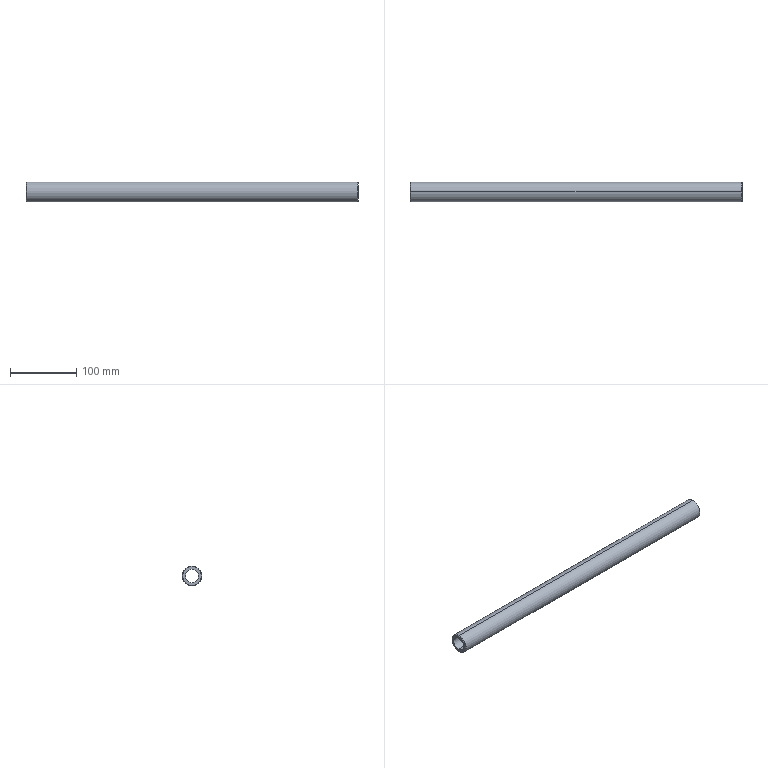Part | STEP file | PSPJ30_X_PSPJ25-400 | 1 solid | 10 faces | box 500 x 30 x 30 mm | volume 196257 mm3 | cone 4 | cylinder 4 | plane 2 | commonest cylinder face diameters 20 x2 30 x2
STEP:
#1=CARTESIAN_POINT('',(0.,0.,0.));
#2=DIRECTION('',(0.,0.,1.));
#3=DIRECTION('',(1.,0.,0.));
#4=AXIS2_PLACEMENT_3D('',#1,#2,#3);
#5=CARTESIAN_POINT('',(0.,0.,14.));
#6=VERTEX_POINT('',#5);
#7=CARTESIAN_POINT('',(0.,0.,-14.));
#8=VERTEX_POINT('',#7);
#9=CARTESIAN_POINT('',(0.,0.,0.));
#10=DIRECTION('',(-1.,0.,0.));
#11=DIRECTION('',(0.,0.,-1.));
#12=AXIS2_PLACEMENT_3D('',#9,#10,#11);
#13=CIRCLE('',#12,14.);
#14=CARTESIAN_POINT('',(0.,0.,0.));
#15=DIRECTION('',(1.,0.,0.));
#16=DIRECTION('',(0.,0.,-1.));
#17=AXIS2_PLACEMENT_3D('',#14,#15,#16);
#18=CONICAL_SURFACE('',#17,14.,0.7854);
#19=CARTESIAN_POINT('',(6.283,0.));
#20=DIRECTION('',(-1.,0.));
#21=VECTOR('',#20,1.);
#22=LINE('',#19,#21);
#23=(GEOMETRIC_REPRESENTATION_CONTEXT(2)PARAMETRIC_REPRESENTATION_CONTEXT()REPRESENTATION_CONTEXT('',''));
#24=DEFINITIONAL_REPRESENTATION('',(#22),#23);
#25=PCURVE('',#18,#24);
#26=CARTESIAN_POINT('',(0.,15.,0.));
#27=DIRECTION('',(1.,0.,0.));
#28=DIRECTION('',(0.,0.,-1.));
#29=AXIS2_PLACEMENT_3D('',#26,#27,#28);
#30=PLANE('',#29);
#31=CARTESIAN_POINT('',(14.,-15.));
#32=CARTESIAN_POINT('',(14.,-39.249));
#33=CARTESIAN_POINT('',(-7.,-27.124));
#34=CARTESIAN_POINT('',(-28.,-15.));
#35=CARTESIAN_POINT('',(-7.,-2.876));
#36=CARTESIAN_POINT('',(14.,9.249));
#37=CARTESIAN_POINT('',(14.,-15.));
#38=(BOUNDED_CURVE()B_SPLINE_CURVE(2,(#31,#32,#33,#34,#35,#36,#37),.UNSPECIFIED.,.T.,.F.)B_SPLINE_CURVE_WITH_KNOTS((1,2,2,2,2,1),(-2.094,0.,2.094,4.189,6.283,8.378),.UNSPECIFIED.)CURVE()GEOMETRIC_REPRESENTATION_ITEM()RATIONAL_B_SPLINE_CURVE((1.,0.5,1.,0.5,1.,0.5,1.))REPRESENTATION_ITEM(''));
#39=(GEOMETRIC_REPRESENTATION_CONTEXT(2)PARAMETRIC_REPRESENTATION_CONTEXT()REPRESENTATION_CONTEXT('',''));
#40=DEFINITIONAL_REPRESENTATION('',(#38),#39);
#41=PCURVE('',#30,#40);
#42=SURFACE_CURVE('',#13,(#25,#41),.PCURVE_S1.);
#43=EDGE_CURVE('',#6,#8,#42,.T.);
#44=ORIENTED_EDGE('',*,*,#43,.F.);
#45=CARTESIAN_POINT('',(1.,0.,15.));
#46=VERTEX_POINT('',#45);
#47=CARTESIAN_POINT('',(0.,0.,14.));
#48=DIRECTION('',(0.7071,0.,0.7071));
#49=VECTOR('',#48,1.);
#50=LINE('',#47,#49);
#51=CARTESIAN_POINT('',(3.142,0.));
#52=DIRECTION('',(0.,1.));
#53=VECTOR('',#52,1.);
#54=LINE('',#51,#53);
#55=(GEOMETRIC_REPRESENTATION_CONTEXT(2)PARAMETRIC_REPRESENTATION_CONTEXT()REPRESENTATION_CONTEXT('',''));
#56=DEFINITIONAL_REPRESENTATION('',(#54),#55);
#57=PCURVE('',#18,#56);
#58=CARTESIAN_POINT('',(0.,0.,0.));
#59=DIRECTION('',(1.,0.,0.));
#60=DIRECTION('',(0.,0.,-1.));
#61=AXIS2_PLACEMENT_3D('',#58,#59,#60);
#62=CONICAL_SURFACE('',#61,14.,0.7854);
#63=CARTESIAN_POINT('',(3.142,0.));
#64=DIRECTION('',(0.,1.));
#65=VECTOR('',#64,1.);
#66=LINE('',#63,#65);
#67=(GEOMETRIC_REPRESENTATION_CONTEXT(2)PARAMETRIC_REPRESENTATION_CONTEXT()REPRESENTATION_CONTEXT('',''));
#68=DEFINITIONAL_REPRESENTATION('',(#66),#67);
#69=PCURVE('',#62,#68);
#70=SURFACE_CURVE('',#50,(#57,#69),.PCURVE_S1.);
#71=EDGE_CURVE('',#6,#46,#70,.T.);
#72=ORIENTED_EDGE('',*,*,#71,.T.);
#73=CARTESIAN_POINT('',(1.,0.,-15.));
#74=VERTEX_POINT('',#73);
#75=CARTESIAN_POINT('',(1.,0.,0.));
#76=DIRECTION('',(1.,0.,0.));
#77=DIRECTION('',(0.,0.,-1.));
#78=AXIS2_PLACEMENT_3D('',#75,#76,#77);
#79=CIRCLE('',#78,15.);
#80=CARTESIAN_POINT('',(0.,1.));
#81=DIRECTION('',(1.,0.));
#82=VECTOR('',#81,1.);
#83=LINE('',#80,#82);
#84=(GEOMETRIC_REPRESENTATION_CONTEXT(2)PARAMETRIC_REPRESENTATION_CONTEXT()REPRESENTATION_CONTEXT('',''));
#85=DEFINITIONAL_REPRESENTATION('',(#83),#84);
#86=PCURVE('',#18,#85);
#87=CARTESIAN_POINT('',(400.,0.,0.));
#88=DIRECTION('',(-1.,0.,0.));
#89=DIRECTION('',(0.,0.,1.));
#90=AXIS2_PLACEMENT_3D('',#87,#88,#89);
#91=CYLINDRICAL_SURFACE('',#90,15.);
#92=CARTESIAN_POINT('',(3.142,399.));
#93=DIRECTION('',(-1.,0.));
#94=VECTOR('',#93,1.);
#95=LINE('',#92,#94);
#96=(GEOMETRIC_REPRESENTATION_CONTEXT(2)PARAMETRIC_REPRESENTATION_CONTEXT()REPRESENTATION_CONTEXT('',''));
#97=DEFINITIONAL_REPRESENTATION('',(#95),#96);
#98=PCURVE('',#91,#97);
#99=SURFACE_CURVE('',#79,(#86,#98),.PCURVE_S1.);
#100=EDGE_CURVE('',#74,#46,#99,.T.);
#101=ORIENTED_EDGE('',*,*,#100,.F.);
#102=CARTESIAN_POINT('',(0.,0.,-14.));
#103=DIRECTION('',(0.7071,0.,-0.7071));
#104=VECTOR('',#103,1.);
#105=LINE('',#102,#104);
#106=CARTESIAN_POINT('',(0.,0.));
#107=DIRECTION('',(0.,1.));
#108=VECTOR('',#107,1.);
#109=LINE('',#106,#108);
#110=(GEOMETRIC_REPRESENTATION_CONTEXT(2)PARAMETRIC_REPRESENTATION_CONTEXT()REPRESENTATION_CONTEXT('',''));
#111=DEFINITIONAL_REPRESENTATION('',(#109),#110);
#112=PCURVE('',#18,#111);
#113=CARTESIAN_POINT('',(6.283,0.));
#114=DIRECTION('',(0.,1.));
#115=VECTOR('',#114,1.);
#116=LINE('',#113,#115);
#117=(GEOMETRIC_REPRESENTATION_CONTEXT(2)PARAMETRIC_REPRESENTATION_CONTEXT()REPRESENTATION_CONTEXT('',''));
#118=DEFINITIONAL_REPRESENTATION('',(#116),#117);
#119=PCURVE('',#62,#118);
#120=SURFACE_CURVE('',#105,(#112,#119),.PCURVE_S1.);
#121=EDGE_CURVE('',#8,#74,#120,.T.);
#122=ORIENTED_EDGE('',*,*,#121,.F.);
#123=EDGE_LOOP('',(#44,#72,#101,#122));
#124=FACE_BOUND('',#123,.T.);
#125=ADVANCED_FACE('',(#124),#18,.T.);
#126=CARTESIAN_POINT('',(500.,0.,-14.));
#127=VERTEX_POINT('',#126);
#128=CARTESIAN_POINT('',(500.,0.,14.));
#129=VERTEX_POINT('',#128);
#130=CARTESIAN_POINT('',(500.,0.,0.));
#131=DIRECTION('',(1.,0.,0.));
#132=DIRECTION('',(0.,0.,1.));
#133=AXIS2_PLACEMENT_3D('',#130,#131,#132);
#134=CIRCLE('',#133,14.);
#135=CARTESIAN_POINT('',(499.,0.,0.));
#136=DIRECTION('',(-1.,0.,0.));
#137=DIRECTION('',(0.,0.,1.));
#138=AXIS2_PLACEMENT_3D('',#135,#136,#137);
#139=CONICAL_SURFACE('',#138,15.,0.7854);
#140=CARTESIAN_POINT('',(6.283,-1.));
#141=DIRECTION('',(-1.,0.));
#142=VECTOR('',#141,1.);
#143=LINE('',#140,#142);
#144=(GEOMETRIC_REPRESENTATION_CONTEXT(2)PARAMETRIC_REPRESENTATION_CONTEXT()REPRESENTATION_CONTEXT('',''));
#145=DEFINITIONAL_REPRESENTATION('',(#143),#144);
#146=PCURVE('',#139,#145);
#147=CARTESIAN_POINT('',(500.,10.,0.));
#148=DIRECTION('',(-1.,0.,0.));
#149=DIRECTION('',(0.,0.,1.));
#150=AXIS2_PLACEMENT_3D('',#147,#148,#149);
#151=PLANE('',#150);
#152=CARTESIAN_POINT('',(14.,-10.));
#153=CARTESIAN_POINT('',(14.,-34.249));
#154=CARTESIAN_POINT('',(-7.,-22.124));
#155=CARTESIAN_POINT('',(-28.,-10.));
#156=CARTESIAN_POINT('',(-7.,2.124));
#157=CARTESIAN_POINT('',(14.,14.249));
#158=CARTESIAN_POINT('',(14.,-10.));
#159=(BOUNDED_CURVE()B_SPLINE_CURVE(2,(#152,#153,#154,#155,#156,#157,#158),.UNSPECIFIED.,.T.,.F.)B_SPLINE_CURVE_WITH_KNOTS((1,2,2,2,2,1),(-2.094,0.,2.094,4.189,6.283,8.378),.UNSPECIFIED.)CURVE()GEOMETRIC_REPRESENTATION_ITEM()RATIONAL_B_SPLINE_CURVE((1.,0.5,1.,0.5,1.,0.5,1.))REPRESENTATION_ITEM(''));
#160=(GEOMETRIC_REPRESENTATION_CONTEXT(2)PARAMETRIC_REPRESENTATION_CONTEXT()REPRESENTATION_CONTEXT('',''));
#161=DEFINITIONAL_REPRESENTATION('',(#159),#160);
#162=PCURVE('',#151,#161);
#163=SURFACE_CURVE('',#134,(#146,#162),.PCURVE_S1.);
#164=EDGE_CURVE('',#127,#129,#163,.T.);
#165=ORIENTED_EDGE('',*,*,#164,.F.);
#166=CARTESIAN_POINT('',(499.,0.,-15.));
#167=VERTEX_POINT('',#166);
#168=CARTESIAN_POINT('',(499.,0.,-15.));
#169=DIRECTION('',(-0.7071,0.,-0.7071));
#170=VECTOR('',#169,1.);
#171=LINE('',#168,#170);
#172=CARTESIAN_POINT('',(3.142,0.));
#173=DIRECTION('',(0.,1.));
#174=VECTOR('',#173,1.);
#175=LINE('',#172,#174);
#176=(GEOMETRIC_REPRESENTATION_CONTEXT(2)PARAMETRIC_REPRESENTATION_CONTEXT()REPRESENTATION_CONTEXT('',''));
#177=DEFINITIONAL_REPRESENTATION('',(#175),#176);
#178=PCURVE('',#139,#177);
#179=CARTESIAN_POINT('',(499.,0.,0.));
#180=DIRECTION('',(-1.,0.,0.));
#181=DIRECTION('',(0.,0.,1.));
#182=AXIS2_PLACEMENT_3D('',#179,#180,#181);
#183=CONICAL_SURFACE('',#182,15.,0.7854);
#184=CARTESIAN_POINT('',(3.142,0.));
#185=DIRECTION('',(0.,1.));
#186=VECTOR('',#185,1.);
#187=LINE('',#184,#186);
#188=(GEOMETRIC_REPRESENTATION_CONTEXT(2)PARAMETRIC_REPRESENTATION_CONTEXT()REPRESENTATION_CONTEXT('',''));
#189=DEFINITIONAL_REPRESENTATION('',(#187),#188);
#190=PCURVE('',#183,#189);
#191=SURFACE_CURVE('',#171,(#178,#190),.PCURVE_S1.);
#192=EDGE_CURVE('',#127,#167,#191,.T.);
#193=ORIENTED_EDGE('',*,*,#192,.T.);
#194=CARTESIAN_POINT('',(499.,0.,15.));
#195=VERTEX_POINT('',#194);
#196=CARTESIAN_POINT('',(499.,0.,0.));
#197=DIRECTION('',(-1.,0.,0.));
#198=DIRECTION('',(0.,0.,1.));
#199=AXIS2_PLACEMENT_3D('',#196,#197,#198);
#200=CIRCLE('',#199,15.);
#201=CARTESIAN_POINT('',(0.,0.));
#202=DIRECTION('',(1.,0.));
#203=VECTOR('',#202,1.);
#204=LINE('',#201,#203);
#205=(GEOMETRIC_REPRESENTATION_CONTEXT(2)PARAMETRIC_REPRESENTATION_CONTEXT()REPRESENTATION_CONTEXT('',''));
#206=DEFINITIONAL_REPRESENTATION('',(#204),#205);
#207=PCURVE('',#139,#206);
#208=CARTESIAN_POINT('',(0.,-99.));
#209=DIRECTION('',(1.,0.));
#210=VECTOR('',#209,1.);
#211=LINE('',#208,#210);
#212=(GEOMETRIC_REPRESENTATION_CONTEXT(2)PARAMETRIC_REPRESENTATION_CONTEXT()REPRESENTATION_CONTEXT('',''));
#213=DEFINITIONAL_REPRESENTATION('',(#211),#212);
#214=PCURVE('',#91,#213);
#215=SURFACE_CURVE('',#200,(#207,#214),.PCURVE_S1.);
#216=EDGE_CURVE('',#195,#167,#215,.T.);
#217=ORIENTED_EDGE('',*,*,#216,.F.);
#218=CARTESIAN_POINT('',(499.,0.,15.));
#219=DIRECTION('',(-0.7071,0.,0.7071));
#220=VECTOR('',#219,1.);
#221=LINE('',#218,#220);
#222=CARTESIAN_POINT('',(0.,0.));
#223=DIRECTION('',(0.,1.));
#224=VECTOR('',#223,1.);
#225=LINE('',#222,#224);
#226=(GEOMETRIC_REPRESENTATION_CONTEXT(2)PARAMETRIC_REPRESENTATION_CONTEXT()REPRESENTATION_CONTEXT('',''));
#227=DEFINITIONAL_REPRESENTATION('',(#225),#226);
#228=PCURVE('',#139,#227);
#229=CARTESIAN_POINT('',(6.283,0.));
#230=DIRECTION('',(0.,1.));
#231=VECTOR('',#230,1.);
#232=LINE('',#229,#231);
#233=(GEOMETRIC_REPRESENTATION_CONTEXT(2)PARAMETRIC_REPRESENTATION_CONTEXT()REPRESENTATION_CONTEXT('',''));
#234=DEFINITIONAL_REPRESENTATION('',(#232),#233);
#235=PCURVE('',#183,#234);
#236=SURFACE_CURVE('',#221,(#228,#235),.PCURVE_S1.);
#237=EDGE_CURVE('',#129,#195,#236,.T.);
#238=ORIENTED_EDGE('',*,*,#237,.F.);
#239=EDGE_LOOP('',(#165,#193,#217,#238));
#240=FACE_BOUND('',#239,.T.);
#241=ADVANCED_FACE('',(#240),#139,.T.);
#242=CARTESIAN_POINT('',(500.,0.,10.));
#243=VERTEX_POINT('',#242);
#244=CARTESIAN_POINT('',(0.,0.,10.));
#245=VERTEX_POINT('',#244);
#246=CARTESIAN_POINT('',(400.,0.,10.));
#247=DIRECTION('',(-1.,0.,0.));
#248=VECTOR('',#247,1.);
#249=LINE('',#246,#248);
#250=CARTESIAN_POINT('',(400.,0.,0.));
#251=DIRECTION('',(-1.,0.,0.));
#252=DIRECTION('',(0.,0.,1.));
#253=AXIS2_PLACEMENT_3D('',#250,#251,#252);
#254=CYLINDRICAL_SURFACE('',#253,10.);
#255=CARTESIAN_POINT('',(6.283,0.));
#256=DIRECTION('',(0.,1.));
#257=VECTOR('',#256,1.);
#258=LINE('',#255,#257);
#259=(GEOMETRIC_REPRESENTATION_CONTEXT(2)PARAMETRIC_REPRESENTATION_CONTEXT()REPRESENTATION_CONTEXT('',''));
#260=DEFINITIONAL_REPRESENTATION('',(#258),#259);
#261=PCURVE('',#254,#260);
#262=CARTESIAN_POINT('',(400.,0.,0.));
#263=DIRECTION('',(-1.,0.,0.));
#264=DIRECTION('',(0.,0.,1.));
#265=AXIS2_PLACEMENT_3D('',#262,#263,#264);
#266=CYLINDRICAL_SURFACE('',#265,10.);
#267=CARTESIAN_POINT('',(0.,0.));
#268=DIRECTION('',(0.,1.));
#269=VECTOR('',#268,1.);
#270=LINE('',#267,#269);
#271=(GEOMETRIC_REPRESENTATION_CONTEXT(2)PARAMETRIC_REPRESENTATION_CONTEXT()REPRESENTATION_CONTEXT('',''));
#272=DEFINITIONAL_REPRESENTATION('',(#270),#271);
#273=PCURVE('',#266,#272);
#274=SURFACE_CURVE('',#249,(#261,#273),.PCURVE_S1.);
#275=EDGE_CURVE('',#243,#245,#274,.T.);
#276=ORIENTED_EDGE('',*,*,#275,.T.);
#277=CARTESIAN_POINT('',(0.,0.,-10.));
#278=VERTEX_POINT('',#277);
#279=CARTESIAN_POINT('',(0.,0.,0.));
#280=DIRECTION('',(-1.,0.,0.));
#281=DIRECTION('',(0.,0.,1.));
#282=AXIS2_PLACEMENT_3D('',#279,#280,#281);
#283=CIRCLE('',#282,10.);
#284=CARTESIAN_POINT('',(0.,400.));
#285=DIRECTION('',(1.,0.));
#286=VECTOR('',#285,1.);
#287=LINE('',#284,#286);
#288=(GEOMETRIC_REPRESENTATION_CONTEXT(2)PARAMETRIC_REPRESENTATION_CONTEXT()REPRESENTATION_CONTEXT('',''));
#289=DEFINITIONAL_REPRESENTATION('',(#287),#288);
#290=PCURVE('',#254,#289);
#291=CARTESIAN_POINT('',(-10.,-15.));
#292=CARTESIAN_POINT('',(-10.,2.321));
#293=CARTESIAN_POINT('',(5.,-6.34));
#294=CARTESIAN_POINT('',(20.,-15.));
#295=CARTESIAN_POINT('',(5.,-23.66));
#296=CARTESIAN_POINT('',(-10.,-32.321));
#297=CARTESIAN_POINT('',(-10.,-15.));
#298=(BOUNDED_CURVE()B_SPLINE_CURVE(2,(#291,#292,#293,#294,#295,#296,#297),.UNSPECIFIED.,.T.,.F.)B_SPLINE_CURVE_WITH_KNOTS((1,2,2,2,2,1),(-2.094,0.,2.094,4.189,6.283,8.378),.UNSPECIFIED.)CURVE()GEOMETRIC_REPRESENTATION_ITEM()RATIONAL_B_SPLINE_CURVE((1.,0.5,1.,0.5,1.,0.5,1.))REPRESENTATION_ITEM(''));
#299=(GEOMETRIC_REPRESENTATION_CONTEXT(2)PARAMETRIC_REPRESENTATION_CONTEXT()REPRESENTATION_CONTEXT('',''));
#300=DEFINITIONAL_REPRESENTATION('',(#298),#299);
#301=PCURVE('',#30,#300);
#302=SURFACE_CURVE('',#283,(#290,#301),.PCURVE_S1.);
#303=EDGE_CURVE('',#278,#245,#302,.T.);
#304=ORIENTED_EDGE('',*,*,#303,.F.);
#305=CARTESIAN_POINT('',(500.,0.,-10.));
#306=VERTEX_POINT('',#305);
#307=CARTESIAN_POINT('',(400.,0.,-10.));
#308=DIRECTION('',(-1.,0.,0.));
#309=VECTOR('',#308,1.);
#310=LINE('',#307,#309);
#311=CARTESIAN_POINT('',(3.142,0.));
#312=DIRECTION('',(0.,1.));
#313=VECTOR('',#312,1.);
#314=LINE('',#311,#313);
#315=(GEOMETRIC_REPRESENTATION_CONTEXT(2)PARAMETRIC_REPRESENTATION_CONTEXT()REPRESENTATION_CONTEXT('',''));
#316=DEFINITIONAL_REPRESENTATION('',(#314),#315);
#317=PCURVE('',#254,#316);
#318=CARTESIAN_POINT('',(3.142,0.));
#319=DIRECTION('',(0.,1.));
#320=VECTOR('',#319,1.);
#321=LINE('',#318,#320);
#322=(GEOMETRIC_REPRESENTATION_CONTEXT(2)PARAMETRIC_REPRESENTATION_CONTEXT()REPRESENTATION_CONTEXT('',''));
#323=DEFINITIONAL_REPRESENTATION('',(#321),#322);
#324=PCURVE('',#266,#323);
#325=SURFACE_CURVE('',#310,(#317,#324),.PCURVE_S1.);
#326=EDGE_CURVE('',#306,#278,#325,.T.);
#327=ORIENTED_EDGE('',*,*,#326,.F.);
#328=CARTESIAN_POINT('',(500.,0.,0.));
#329=DIRECTION('',(-1.,0.,0.));
#330=DIRECTION('',(0.,0.,1.));
#331=AXIS2_PLACEMENT_3D('',#328,#329,#330);
#332=CIRCLE('',#331,10.);
#333=CARTESIAN_POINT('',(0.,-100.));
#334=DIRECTION('',(1.,0.));
#335=VECTOR('',#334,1.);
#336=LINE('',#333,#335);
#337=(GEOMETRIC_REPRESENTATION_CONTEXT(2)PARAMETRIC_REPRESENTATION_CONTEXT()REPRESENTATION_CONTEXT('',''));
#338=DEFINITIONAL_REPRESENTATION('',(#336),#337);
#339=PCURVE('',#254,#338);
#340=CARTESIAN_POINT('',(0.,-10.));
#341=DIRECTION('',(1.,0.));
#342=AXIS2_PLACEMENT_2D('',#340,#341);
#343=CIRCLE('',#342,10.);
#344=(GEOMETRIC_REPRESENTATION_CONTEXT(2)PARAMETRIC_REPRESENTATION_CONTEXT()REPRESENTATION_CONTEXT('',''));
#345=DEFINITIONAL_REPRESENTATION('',(#343),#344);
#346=PCURVE('',#151,#345);
#347=SURFACE_CURVE('',#332,(#339,#346),.PCURVE_S1.);
#348=EDGE_CURVE('',#306,#243,#347,.T.);
#349=ORIENTED_EDGE('',*,*,#348,.T.);
#350=EDGE_LOOP('',(#276,#304,#327,#349));
#351=FACE_BOUND('',#350,.F.);
#352=ADVANCED_FACE('',(#351),#254,.F.);
#353=ORIENTED_EDGE('',*,*,#216,.T.);
#354=CARTESIAN_POINT('',(400.,0.,-15.));
#355=DIRECTION('',(-1.,0.,0.));
#356=VECTOR('',#355,1.);
#357=LINE('',#354,#356);
#358=CARTESIAN_POINT('',(3.142,0.));
#359=DIRECTION('',(0.,1.));
#360=VECTOR('',#359,1.);
#361=LINE('',#358,#360);
#362=(GEOMETRIC_REPRESENTATION_CONTEXT(2)PARAMETRIC_REPRESENTATION_CONTEXT()REPRESENTATION_CONTEXT('',''));
#363=DEFINITIONAL_REPRESENTATION('',(#361),#362);
#364=PCURVE('',#91,#363);
#365=CARTESIAN_POINT('',(400.,0.,0.));
#366=DIRECTION('',(-1.,0.,0.));
#367=DIRECTION('',(0.,0.,1.));
#368=AXIS2_PLACEMENT_3D('',#365,#366,#367);
#369=CYLINDRICAL_SURFACE('',#368,15.);
#370=CARTESIAN_POINT('',(3.142,0.));
#371=DIRECTION('',(0.,1.));
#372=VECTOR('',#371,1.);
#373=LINE('',#370,#372);
#374=(GEOMETRIC_REPRESENTATION_CONTEXT(2)PARAMETRIC_REPRESENTATION_CONTEXT()REPRESENTATION_CONTEXT('',''));
#375=DEFINITIONAL_REPRESENTATION('',(#373),#374);
#376=PCURVE('',#369,#375);
#377=SURFACE_CURVE('',#357,(#364,#376),.PCURVE_S1.);
#378=EDGE_CURVE('',#167,#74,#377,.T.);
#379=ORIENTED_EDGE('',*,*,#378,.T.);
#380=ORIENTED_EDGE('',*,*,#100,.T.);
#381=CARTESIAN_POINT('',(400.,0.,15.));
#382=DIRECTION('',(-1.,0.,0.));
#383=VECTOR('',#382,1.);
#384=LINE('',#381,#383);
#385=CARTESIAN_POINT('',(0.,0.));
#386=DIRECTION('',(0.,1.));
#387=VECTOR('',#386,1.);
#388=LINE('',#385,#387);
#389=(GEOMETRIC_REPRESENTATION_CONTEXT(2)PARAMETRIC_REPRESENTATION_CONTEXT()REPRESENTATION_CONTEXT('',''));
#390=DEFINITIONAL_REPRESENTATION('',(#388),#389);
#391=PCURVE('',#91,#390);
#392=CARTESIAN_POINT('',(6.283,0.));
#393=DIRECTION('',(0.,1.));
#394=VECTOR('',#393,1.);
#395=LINE('',#392,#394);
#396=(GEOMETRIC_REPRESENTATION_CONTEXT(2)PARAMETRIC_REPRESENTATION_CONTEXT()REPRESENTATION_CONTEXT('',''));
#397=DEFINITIONAL_REPRESENTATION('',(#395),#396);
#398=PCURVE('',#369,#397);
#399=SURFACE_CURVE('',#384,(#391,#398),.PCURVE_S1.);
#400=EDGE_CURVE('',#195,#46,#399,.T.);
#401=ORIENTED_EDGE('',*,*,#400,.F.);
#402=EDGE_LOOP('',(#353,#379,#380,#401));
#403=FACE_BOUND('',#402,.T.);
#404=ADVANCED_FACE('',(#403),#91,.T.);
#405=ORIENTED_EDGE('',*,*,#378,.F.);
#406=CARTESIAN_POINT('',(499.,0.,0.));
#407=DIRECTION('',(-1.,0.,0.));
#408=DIRECTION('',(0.,0.,1.));
#409=AXIS2_PLACEMENT_3D('',#406,#407,#408);
#410=CIRCLE('',#409,15.);
#411=CARTESIAN_POINT('',(0.,-99.));
#412=DIRECTION('',(1.,0.));
#413=VECTOR('',#412,1.);
#414=LINE('',#411,#413);
#415=(GEOMETRIC_REPRESENTATION_CONTEXT(2)PARAMETRIC_REPRESENTATION_CONTEXT()REPRESENTATION_CONTEXT('',''));
#416=DEFINITIONAL_REPRESENTATION('',(#414),#415);
#417=PCURVE('',#369,#416);
#418=CARTESIAN_POINT('',(0.,0.));
#419=DIRECTION('',(1.,0.));
#420=VECTOR('',#419,1.);
#421=LINE('',#418,#420);
#422=(GEOMETRIC_REPRESENTATION_CONTEXT(2)PARAMETRIC_REPRESENTATION_CONTEXT()REPRESENTATION_CONTEXT('',''));
#423=DEFINITIONAL_REPRESENTATION('',(#421),#422);
#424=PCURVE('',#183,#423);
#425=SURFACE_CURVE('',#410,(#417,#424),.PCURVE_S1.);
#426=EDGE_CURVE('',#167,#195,#425,.T.);
#427=ORIENTED_EDGE('',*,*,#426,.T.);
#428=ORIENTED_EDGE('',*,*,#400,.T.);
#429=CARTESIAN_POINT('',(1.,0.,0.));
#430=DIRECTION('',(1.,0.,0.));
#431=DIRECTION('',(0.,0.,-1.));
#432=AXIS2_PLACEMENT_3D('',#429,#430,#431);
#433=CIRCLE('',#432,15.);
#434=CARTESIAN_POINT('',(9.425,399.));
#435=DIRECTION('',(-1.,0.));
#436=VECTOR('',#435,1.);
#437=LINE('',#434,#436);
#438=(GEOMETRIC_REPRESENTATION_CONTEXT(2)PARAMETRIC_REPRESENTATION_CONTEXT()REPRESENTATION_CONTEXT('',''));
#439=DEFINITIONAL_REPRESENTATION('',(#437),#438);
#440=PCURVE('',#369,#439);
#441=CARTESIAN_POINT('',(0.,1.));
#442=DIRECTION('',(1.,0.));
#443=VECTOR('',#442,1.);
#444=LINE('',#441,#443);
#445=(GEOMETRIC_REPRESENTATION_CONTEXT(2)PARAMETRIC_REPRESENTATION_CONTEXT()REPRESENTATION_CONTEXT('',''));
#446=DEFINITIONAL_REPRESENTATION('',(#444),#445);
#447=PCURVE('',#62,#446);
#448=SURFACE_CURVE('',#433,(#440,#447),.PCURVE_S1.);
#449=EDGE_CURVE('',#46,#74,#448,.T.);
#450=ORIENTED_EDGE('',*,*,#449,.T.);
#451=EDGE_LOOP('',(#405,#427,#428,#450));
#452=FACE_BOUND('',#451,.T.);
#453=ADVANCED_FACE('',(#452),#369,.T.);
#454=CARTESIAN_POINT('',(0.,0.,0.));
#455=DIRECTION('',(-1.,0.,0.));
#456=DIRECTION('',(0.,0.,-1.));
#457=AXIS2_PLACEMENT_3D('',#454,#455,#456);
#458=CIRCLE('',#457,14.);
#459=CARTESIAN_POINT('',(14.,-15.));
#460=CARTESIAN_POINT('',(14.,-39.249));
#461=CARTESIAN_POINT('',(-7.,-27.124));
#462=CARTESIAN_POINT('',(-28.,-15.));
#463=CARTESIAN_POINT('',(-7.,-2.876));
#464=CARTESIAN_POINT('',(14.,9.249));
#465=CARTESIAN_POINT('',(14.,-15.));
#466=(BOUNDED_CURVE()B_SPLINE_CURVE(2,(#459,#460,#461,#462,#463,#464,#465),.UNSPECIFIED.,.T.,.F.)B_SPLINE_CURVE_WITH_KNOTS((1,2,2,2,2,1),(-2.094,0.,2.094,4.189,6.283,8.378),.UNSPECIFIED.)CURVE()GEOMETRIC_REPRESENTATION_ITEM()RATIONAL_B_SPLINE_CURVE((1.,0.5,1.,0.5,1.,0.5,1.))REPRESENTATION_ITEM(''));
#467=(GEOMETRIC_REPRESENTATION_CONTEXT(2)PARAMETRIC_REPRESENTATION_CONTEXT()REPRESENTATION_CONTEXT('',''));
#468=DEFINITIONAL_REPRESENTATION('',(#466),#467);
#469=PCURVE('',#30,#468);
#470=CARTESIAN_POINT('',(6.283,0.));
#471=DIRECTION('',(-1.,0.));
#472=VECTOR('',#471,1.);
#473=LINE('',#470,#472);
#474=(GEOMETRIC_REPRESENTATION_CONTEXT(2)PARAMETRIC_REPRESENTATION_CONTEXT()REPRESENTATION_CONTEXT('',''));
#475=DEFINITIONAL_REPRESENTATION('',(#473),#474);
#476=PCURVE('',#62,#475);
#477=SURFACE_CURVE('',#458,(#469,#476),.PCURVE_S1.);
#478=EDGE_CURVE('',#8,#6,#477,.T.);
#479=ORIENTED_EDGE('',*,*,#478,.T.);
#480=ORIENTED_EDGE('',*,*,#43,.T.);
#481=EDGE_LOOP('',(#479,#480));
#482=FACE_BOUND('',#481,.T.);
#483=CARTESIAN_POINT('',(0.,0.,0.));
#484=DIRECTION('',(-1.,0.,0.));
#485=DIRECTION('',(0.,0.,1.));
#486=AXIS2_PLACEMENT_3D('',#483,#484,#485);
#487=CIRCLE('',#486,10.);
#488=CARTESIAN_POINT('',(-10.,-15.));
#489=CARTESIAN_POINT('',(-10.,2.321));
#490=CARTESIAN_POINT('',(5.,-6.34));
#491=CARTESIAN_POINT('',(20.,-15.));
#492=CARTESIAN_POINT('',(5.,-23.66));
#493=CARTESIAN_POINT('',(-10.,-32.321));
#494=CARTESIAN_POINT('',(-10.,-15.));
#495=(BOUNDED_CURVE()B_SPLINE_CURVE(2,(#488,#489,#490,#491,#492,#493,#494),.UNSPECIFIED.,.T.,.F.)B_SPLINE_CURVE_WITH_KNOTS((1,2,2,2,2,1),(-2.094,0.,2.094,4.189,6.283,8.378),.UNSPECIFIED.)CURVE()GEOMETRIC_REPRESENTATION_ITEM()RATIONAL_B_SPLINE_CURVE((1.,0.5,1.,0.5,1.,0.5,1.))REPRESENTATION_ITEM(''));
#496=(GEOMETRIC_REPRESENTATION_CONTEXT(2)PARAMETRIC_REPRESENTATION_CONTEXT()REPRESENTATION_CONTEXT('',''));
#497=DEFINITIONAL_REPRESENTATION('',(#495),#496);
#498=PCURVE('',#30,#497);
#499=CARTESIAN_POINT('',(0.,400.));
#500=DIRECTION('',(1.,0.));
#501=VECTOR('',#500,1.);
#502=LINE('',#499,#501);
#503=(GEOMETRIC_REPRESENTATION_CONTEXT(2)PARAMETRIC_REPRESENTATION_CONTEXT()REPRESENTATION_CONTEXT('',''));
#504=DEFINITIONAL_REPRESENTATION('',(#502),#503);
#505=PCURVE('',#266,#504);
#506=SURFACE_CURVE('',#487,(#498,#505),.PCURVE_S1.);
#507=EDGE_CURVE('',#245,#278,#506,.T.);
#508=ORIENTED_EDGE('',*,*,#507,.F.);
#509=ORIENTED_EDGE('',*,*,#303,.F.);
#510=EDGE_LOOP('',(#508,#509));
#511=FACE_BOUND('',#510,.T.);
#512=ADVANCED_FACE('',(#482,#511),#30,.F.);
#513=ORIENTED_EDGE('',*,*,#507,.F.);
#514=ORIENTED_EDGE('',*,*,#275,.F.);
#515=CARTESIAN_POINT('',(500.,0.,0.));
#516=DIRECTION('',(-1.,0.,0.));
#517=DIRECTION('',(0.,0.,1.));
#518=AXIS2_PLACEMENT_3D('',#515,#516,#517);
#519=CIRCLE('',#518,10.);
#520=CARTESIAN_POINT('',(0.,-100.));
#521=DIRECTION('',(1.,0.));
#522=VECTOR('',#521,1.);
#523=LINE('',#520,#522);
#524=(GEOMETRIC_REPRESENTATION_CONTEXT(2)PARAMETRIC_REPRESENTATION_CONTEXT()REPRESENTATION_CONTEXT('',''));
#525=DEFINITIONAL_REPRESENTATION('',(#523),#524);
#526=PCURVE('',#266,#525);
#527=CARTESIAN_POINT('',(0.,-10.));
#528=DIRECTION('',(1.,0.));
#529=AXIS2_PLACEMENT_2D('',#527,#528);
#530=CIRCLE('',#529,10.);
#531=(GEOMETRIC_REPRESENTATION_CONTEXT(2)PARAMETRIC_REPRESENTATION_CONTEXT()REPRESENTATION_CONTEXT('',''));
#532=DEFINITIONAL_REPRESENTATION('',(#530),#531);
#533=PCURVE('',#151,#532);
#534=SURFACE_CURVE('',#519,(#526,#533),.PCURVE_S1.);
#535=EDGE_CURVE('',#243,#306,#534,.T.);
#536=ORIENTED_EDGE('',*,*,#535,.T.);
#537=ORIENTED_EDGE('',*,*,#326,.T.);
#538=EDGE_LOOP('',(#513,#514,#536,#537));
#539=FACE_BOUND('',#538,.F.);
#540=ADVANCED_FACE('',(#539),#266,.F.);
#541=CARTESIAN_POINT('',(500.,0.,0.));
#542=DIRECTION('',(1.,0.,0.));
#543=DIRECTION('',(0.,0.,1.));
#544=AXIS2_PLACEMENT_3D('',#541,#542,#543);
#545=CIRCLE('',#544,14.);
#546=CARTESIAN_POINT('',(14.,-10.));
#547=CARTESIAN_POINT('',(14.,-34.249));
#548=CARTESIAN_POINT('',(-7.,-22.124));
#549=CARTESIAN_POINT('',(-28.,-10.));
#550=CARTESIAN_POINT('',(-7.,2.124));
#551=CARTESIAN_POINT('',(14.,14.249));
#552=CARTESIAN_POINT('',(14.,-10.));
#553=(BOUNDED_CURVE()B_SPLINE_CURVE(2,(#546,#547,#548,#549,#550,#551,#552),.UNSPECIFIED.,.T.,.F.)B_SPLINE_CURVE_WITH_KNOTS((1,2,2,2,2,1),(-2.094,0.,2.094,4.189,6.283,8.378),.UNSPECIFIED.)CURVE()GEOMETRIC_REPRESENTATION_ITEM()RATIONAL_B_SPLINE_CURVE((1.,0.5,1.,0.5,1.,0.5,1.))REPRESENTATION_ITEM(''));
#554=(GEOMETRIC_REPRESENTATION_CONTEXT(2)PARAMETRIC_REPRESENTATION_CONTEXT()REPRESENTATION_CONTEXT('',''));
#555=DEFINITIONAL_REPRESENTATION('',(#553),#554);
#556=PCURVE('',#151,#555);
#557=CARTESIAN_POINT('',(6.283,-1.));
#558=DIRECTION('',(-1.,0.));
#559=VECTOR('',#558,1.);
#560=LINE('',#557,#559);
#561=(GEOMETRIC_REPRESENTATION_CONTEXT(2)PARAMETRIC_REPRESENTATION_CONTEXT()REPRESENTATION_CONTEXT('',''));
#562=DEFINITIONAL_REPRESENTATION('',(#560),#561);
#563=PCURVE('',#183,#562);
#564=SURFACE_CURVE('',#545,(#556,#563),.PCURVE_S1.);
#565=EDGE_CURVE('',#129,#127,#564,.T.);
#566=ORIENTED_EDGE('',*,*,#565,.T.);
#567=ORIENTED_EDGE('',*,*,#164,.T.);
#568=EDGE_LOOP('',(#566,#567));
#569=FACE_BOUND('',#568,.T.);
#570=ORIENTED_EDGE('',*,*,#535,.T.);
#571=ORIENTED_EDGE('',*,*,#348,.T.);
#572=EDGE_LOOP('',(#570,#571));
#573=FACE_BOUND('',#572,.T.);
#574=ADVANCED_FACE('',(#569,#573),#151,.F.);
#575=ORIENTED_EDGE('',*,*,#192,.F.);
#576=ORIENTED_EDGE('',*,*,#565,.F.);
#577=ORIENTED_EDGE('',*,*,#237,.T.);
#578=ORIENTED_EDGE('',*,*,#426,.F.);
#579=EDGE_LOOP('',(#575,#576,#577,#578));
#580=FACE_BOUND('',#579,.T.);
#581=ADVANCED_FACE('',(#580),#183,.T.);
#582=ORIENTED_EDGE('',*,*,#71,.F.);
#583=ORIENTED_EDGE('',*,*,#478,.F.);
#584=ORIENTED_EDGE('',*,*,#121,.T.);
#585=ORIENTED_EDGE('',*,*,#449,.F.);
#586=EDGE_LOOP('',(#582,#583,#584,#585));
#587=FACE_BOUND('',#586,.T.);
#588=ADVANCED_FACE('',(#587),#62,.T.);
#589=CLOSED_SHELL('',(#125,#241,#352,#404,#453,#512,#540,#574,#581,#588));
#590=MANIFOLD_SOLID_BREP('',#589);
#591=(LENGTH_UNIT()NAMED_UNIT(*)SI_UNIT(.MILLI.,.METRE.));
#592=UNCERTAINTY_MEASURE_WITH_UNIT(LENGTH_MEASURE(0.0000001),#591,'','');
#593=(NAMED_UNIT(*)PLANE_ANGLE_UNIT()SI_UNIT($,.RADIAN.));
#594=(NAMED_UNIT(*)SI_UNIT($,.STERADIAN.)SOLID_ANGLE_UNIT());
#595=(GEOMETRIC_REPRESENTATION_CONTEXT(3)GLOBAL_UNCERTAINTY_ASSIGNED_CONTEXT((#592))GLOBAL_UNIT_ASSIGNED_CONTEXT((#591,#593,#594))REPRESENTATION_CONTEXT('',''));
#596=ADVANCED_BREP_SHAPE_REPRESENTATION('',(#4,#590),#595);